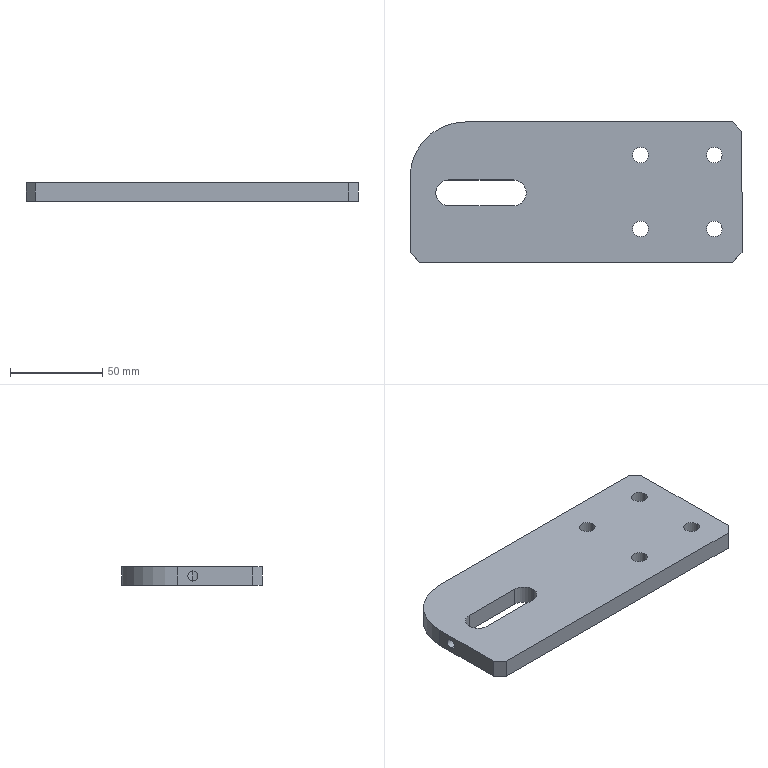Part | SolidWorks | features HoleWzd 2, Chamfer 1, Extrusion 1, ICE 1, LPattern 1, MirrorPattern 1 | 1 solid | 25 faces | box 180 x 76 x 10 mm | volume 125449 mm3 | cylinder 14 | plane 11 | commonest cylinder face diameters 8.5 x8 14 x3 5.5 x2 60 x1
STEP:
#1=CARTESIAN_POINT('',(-76.,-0.5,-2.75));
#2=VERTEX_POINT('',#1);
#3=CARTESIAN_POINT('',(-76.,-0.5,2.75));
#4=VERTEX_POINT('',#3);
#5=CARTESIAN_POINT('',(-76.,-0.5,-2.75));
#6=CARTESIAN_POINT('',(-76.,-0.6808,-2.75));
#7=CARTESIAN_POINT('',(-75.993,-0.8639,-2.732));
#8=CARTESIAN_POINT('',(-75.965,-1.22,-2.66));
#9=CARTESIAN_POINT('',(-75.945,-1.392,-2.607));
#10=CARTESIAN_POINT('',(-75.894,-1.725,-2.469));
#11=CARTESIAN_POINT('',(-75.863,-1.885,-2.382));
#12=CARTESIAN_POINT('',(-75.797,-2.181,-2.184));
#13=CARTESIAN_POINT('',(-75.761,-2.319,-2.071));
#14=CARTESIAN_POINT('',(-75.687,-2.572,-1.817));
#15=CARTESIAN_POINT('',(-75.651,-2.685,-1.679));
#16=CARTESIAN_POINT('',(-75.583,-2.883,-1.384));
#17=CARTESIAN_POINT('',(-75.551,-2.969,-1.224));
#18=CARTESIAN_POINT('',(-75.497,-3.107,-0.8921));
#19=CARTESIAN_POINT('',(-75.475,-3.16,-0.7207));
#20=CARTESIAN_POINT('',(-75.445,-3.231,-0.3666));
#21=CARTESIAN_POINT('',(-75.437,-3.25,-0.1823));
#22=CARTESIAN_POINT('',(-75.437,-3.25,0.18));
#23=CARTESIAN_POINT('',(-75.445,-3.232,0.3601));
#24=CARTESIAN_POINT('',(-75.475,-3.161,0.7177));
#25=CARTESIAN_POINT('',(-75.497,-3.108,0.8913));
#26=CARTESIAN_POINT('',(-75.55,-2.97,1.222));
#27=CARTESIAN_POINT('',(-75.582,-2.884,1.382));
#28=CARTESIAN_POINT('',(-75.651,-2.685,1.679));
#29=CARTESIAN_POINT('',(-75.688,-2.572,1.817));
#30=CARTESIAN_POINT('',(-75.76,-2.32,2.069));
#31=CARTESIAN_POINT('',(-75.797,-2.181,2.184));
#32=CARTESIAN_POINT('',(-75.863,-1.885,2.382));
#33=CARTESIAN_POINT('',(-75.893,-1.728,2.467));
#34=CARTESIAN_POINT('',(-75.97,-1.227,2.677));
#35=CARTESIAN_POINT('',(-76.,-0.8671,2.75));
#36=CARTESIAN_POINT('',(-76.,-0.5,2.75));
#37=B_SPLINE_CURVE_WITH_KNOTS('',3,(#5,#6,#7,#8,#9,#10,#11,#12,#13,#14,#15,#16,#17,#18,#19,#20,#21,#22,#23,#24,#25,#26,#27,#28,#29,#30,#31,#32,#33,#34,#35,#36),.UNSPECIFIED.,.F.,.F.,(4,2,2,2,2,2,2,2,2,2,2,2,2,2,2,4),(0.008686,0.009229,0.009771,0.01031,0.01086,0.0114,0.01194,0.01248,0.01303,0.01357,0.01411,0.01465,0.0152,0.01574,0.01628,0.01737),.UNSPECIFIED.);
#38=EDGE_CURVE('',#2,#4,#37,.T.);
#39=ORIENTED_EDGE('',*,*,#38,.F.);
#40=CARTESIAN_POINT('',(-90.,-0.5,-2.75));
#41=VERTEX_POINT('',#40);
#42=CARTESIAN_POINT('',(-90.,-0.5,-2.75));
#43=DIRECTION('',(-1.,0.,0.));
#44=VECTOR('',#43,1000.);
#45=LINE('',#42,#44);
#46=EDGE_CURVE('',#2,#41,#45,.T.);
#47=ORIENTED_EDGE('',*,*,#46,.T.);
#48=CARTESIAN_POINT('',(-90.,-0.5,2.75));
#49=VERTEX_POINT('',#48);
#50=CARTESIAN_POINT('',(-90.,-0.5,0.));
#51=DIRECTION('',(-1.,0.,0.));
#52=DIRECTION('',(0.,0.,1.));
#53=AXIS2_PLACEMENT_3D('',#50,#51,#52);
#54=CIRCLE('',#53,2.75);
#55=EDGE_CURVE('',#41,#49,#54,.T.);
#56=ORIENTED_EDGE('',*,*,#55,.T.);
#57=CARTESIAN_POINT('',(-90.,-0.5,2.75));
#58=DIRECTION('',(-1.,0.,0.));
#59=VECTOR('',#58,1000.);
#60=LINE('',#57,#59);
#61=EDGE_CURVE('',#4,#49,#60,.T.);
#62=ORIENTED_EDGE('',*,*,#61,.F.);
#63=EDGE_LOOP('',(#39,#47,#56,#62));
#64=FACE_OUTER_BOUND('',#63,.T.);
#65=CARTESIAN_POINT('',(-90.,-0.5,0.));
#66=DIRECTION('',(-1.,0.,0.));
#67=DIRECTION('',(0.,0.,1.));
#68=AXIS2_PLACEMENT_3D('',#65,#66,#67);
#69=CYLINDRICAL_SURFACE('',#68,2.75);
#70=ADVANCED_FACE('',(#64),#69,.F.);
#71=CARTESIAN_POINT('',(-27.,-0.5,-5.));
#72=VERTEX_POINT('',#71);
#73=CARTESIAN_POINT('',(-34.,6.5,-5.));
#74=VERTEX_POINT('',#73);
#75=CARTESIAN_POINT('',(-34.,-0.5,-5.));
#76=DIRECTION('',(0.,0.,1.));
#77=DIRECTION('',(1.,0.,0.));
#78=AXIS2_PLACEMENT_3D('',#75,#76,#77);
#79=CIRCLE('',#78,7.);
#80=EDGE_CURVE('',#72,#74,#79,.T.);
#81=ORIENTED_EDGE('',*,*,#80,.F.);
#82=CARTESIAN_POINT('',(-27.,-0.5,5.));
#83=VERTEX_POINT('',#82);
#84=CARTESIAN_POINT('',(-27.,-0.5,-5.));
#85=DIRECTION('',(0.,0.,1.));
#86=VECTOR('',#85,1000.);
#87=LINE('',#84,#86);
#88=EDGE_CURVE('',#72,#83,#87,.T.);
#89=ORIENTED_EDGE('',*,*,#88,.T.);
#90=CARTESIAN_POINT('',(-34.,6.5,5.));
#91=VERTEX_POINT('',#90);
#92=CARTESIAN_POINT('',(-34.,-0.5,5.));
#93=DIRECTION('',(0.,0.,1.));
#94=DIRECTION('',(1.,0.,0.));
#95=AXIS2_PLACEMENT_3D('',#92,#93,#94);
#96=CIRCLE('',#95,7.);
#97=EDGE_CURVE('',#83,#91,#96,.T.);
#98=ORIENTED_EDGE('',*,*,#97,.T.);
#99=CARTESIAN_POINT('',(-34.,6.5,-5.));
#100=DIRECTION('',(0.,0.,1.));
#101=VECTOR('',#100,1000.);
#102=LINE('',#99,#101);
#103=EDGE_CURVE('',#74,#91,#102,.T.);
#104=ORIENTED_EDGE('',*,*,#103,.F.);
#105=EDGE_LOOP('',(#81,#89,#98,#104));
#106=FACE_OUTER_BOUND('',#105,.T.);
#107=CARTESIAN_POINT('',(-34.,-0.5,-5.));
#108=DIRECTION('',(0.,0.,1.));
#109=DIRECTION('',(1.,0.,0.));
#110=AXIS2_PLACEMENT_3D('',#107,#108,#109);
#111=CYLINDRICAL_SURFACE('',#110,7.);
#112=ADVANCED_FACE('',(#106),#111,.F.);
#113=CARTESIAN_POINT('',(30.75,-20.,-5.));
#114=VERTEX_POINT('',#113);
#115=CARTESIAN_POINT('',(39.25,-20.,-5.));
#116=VERTEX_POINT('',#115);
#117=CARTESIAN_POINT('',(35.,-20.,-5.));
#118=DIRECTION('',(0.,0.,1.));
#119=DIRECTION('',(1.,0.,0.));
#120=AXIS2_PLACEMENT_3D('',#117,#118,#119);
#121=CIRCLE('',#120,4.25);
#122=EDGE_CURVE('',#114,#116,#121,.T.);
#123=ORIENTED_EDGE('',*,*,#122,.F.);
#124=CARTESIAN_POINT('',(30.75,-20.,5.));
#125=VERTEX_POINT('',#124);
#126=CARTESIAN_POINT('',(30.75,-20.,5.));
#127=DIRECTION('',(0.,0.,1.));
#128=VECTOR('',#127,1000.);
#129=LINE('',#126,#128);
#130=EDGE_CURVE('',#114,#125,#129,.T.);
#131=ORIENTED_EDGE('',*,*,#130,.T.);
#132=CARTESIAN_POINT('',(39.25,-20.,5.));
#133=VERTEX_POINT('',#132);
#134=CARTESIAN_POINT('',(35.,-20.,5.));
#135=DIRECTION('',(0.,0.,1.));
#136=DIRECTION('',(1.,0.,0.));
#137=AXIS2_PLACEMENT_3D('',#134,#135,#136);
#138=CIRCLE('',#137,4.25);
#139=EDGE_CURVE('',#125,#133,#138,.T.);
#140=ORIENTED_EDGE('',*,*,#139,.T.);
#141=CARTESIAN_POINT('',(39.25,-20.,5.));
#142=DIRECTION('',(0.,0.,1.));
#143=VECTOR('',#142,1000.);
#144=LINE('',#141,#143);
#145=EDGE_CURVE('',#116,#133,#144,.T.);
#146=ORIENTED_EDGE('',*,*,#145,.F.);
#147=EDGE_LOOP('',(#123,#131,#140,#146));
#148=FACE_OUTER_BOUND('',#147,.T.);
#149=CARTESIAN_POINT('',(35.,-20.,5.));
#150=DIRECTION('',(0.,0.,1.));
#151=DIRECTION('',(1.,0.,0.));
#152=AXIS2_PLACEMENT_3D('',#149,#150,#151);
#153=CYLINDRICAL_SURFACE('',#152,4.25);
#154=ADVANCED_FACE('',(#148),#153,.F.);
#155=CARTESIAN_POINT('',(70.75,-20.,-5.));
#156=VERTEX_POINT('',#155);
#157=CARTESIAN_POINT('',(79.25,-20.,-5.));
#158=VERTEX_POINT('',#157);
#159=CARTESIAN_POINT('',(75.,-20.,-5.));
#160=DIRECTION('',(0.,0.,1.));
#161=DIRECTION('',(1.,0.,0.));
#162=AXIS2_PLACEMENT_3D('',#159,#160,#161);
#163=CIRCLE('',#162,4.25);
#164=EDGE_CURVE('',#156,#158,#163,.T.);
#165=ORIENTED_EDGE('',*,*,#164,.F.);
#166=CARTESIAN_POINT('',(70.75,-20.,5.));
#167=VERTEX_POINT('',#166);
#168=CARTESIAN_POINT('',(70.75,-20.,5.));
#169=DIRECTION('',(0.,0.,1.));
#170=VECTOR('',#169,1000.);
#171=LINE('',#168,#170);
#172=EDGE_CURVE('',#156,#167,#171,.T.);
#173=ORIENTED_EDGE('',*,*,#172,.T.);
#174=CARTESIAN_POINT('',(79.25,-20.,5.));
#175=VERTEX_POINT('',#174);
#176=CARTESIAN_POINT('',(75.,-20.,5.));
#177=DIRECTION('',(0.,0.,1.));
#178=DIRECTION('',(1.,0.,0.));
#179=AXIS2_PLACEMENT_3D('',#176,#177,#178);
#180=CIRCLE('',#179,4.25);
#181=EDGE_CURVE('',#167,#175,#180,.T.);
#182=ORIENTED_EDGE('',*,*,#181,.T.);
#183=CARTESIAN_POINT('',(79.25,-20.,5.));
#184=DIRECTION('',(0.,0.,1.));
#185=VECTOR('',#184,1000.);
#186=LINE('',#183,#185);
#187=EDGE_CURVE('',#158,#175,#186,.T.);
#188=ORIENTED_EDGE('',*,*,#187,.F.);
#189=EDGE_LOOP('',(#165,#173,#182,#188));
#190=FACE_OUTER_BOUND('',#189,.T.);
#191=CARTESIAN_POINT('',(75.,-20.,5.));
#192=DIRECTION('',(0.,0.,1.));
#193=DIRECTION('',(1.,0.,0.));
#194=AXIS2_PLACEMENT_3D('',#191,#192,#193);
#195=CYLINDRICAL_SURFACE('',#194,4.25);
#196=ADVANCED_FACE('',(#190),#195,.F.);
#197=CARTESIAN_POINT('',(30.75,20.,-5.));
#198=VERTEX_POINT('',#197);
#199=CARTESIAN_POINT('',(39.25,20.,-5.));
#200=VERTEX_POINT('',#199);
#201=CARTESIAN_POINT('',(35.,20.,-5.));
#202=DIRECTION('',(0.,0.,1.));
#203=DIRECTION('',(1.,0.,0.));
#204=AXIS2_PLACEMENT_3D('',#201,#202,#203);
#205=CIRCLE('',#204,4.25);
#206=EDGE_CURVE('',#198,#200,#205,.T.);
#207=ORIENTED_EDGE('',*,*,#206,.F.);
#208=CARTESIAN_POINT('',(30.75,20.,5.));
#209=VERTEX_POINT('',#208);
#210=CARTESIAN_POINT('',(30.75,20.,5.));
#211=DIRECTION('',(0.,0.,1.));
#212=VECTOR('',#211,1000.);
#213=LINE('',#210,#212);
#214=EDGE_CURVE('',#198,#209,#213,.T.);
#215=ORIENTED_EDGE('',*,*,#214,.T.);
#216=CARTESIAN_POINT('',(39.25,20.,5.));
#217=VERTEX_POINT('',#216);
#218=CARTESIAN_POINT('',(35.,20.,5.));
#219=DIRECTION('',(0.,0.,1.));
#220=DIRECTION('',(1.,0.,0.));
#221=AXIS2_PLACEMENT_3D('',#218,#219,#220);
#222=CIRCLE('',#221,4.25);
#223=EDGE_CURVE('',#209,#217,#222,.T.);
#224=ORIENTED_EDGE('',*,*,#223,.T.);
#225=CARTESIAN_POINT('',(39.25,20.,5.));
#226=DIRECTION('',(0.,0.,1.));
#227=VECTOR('',#226,1000.);
#228=LINE('',#225,#227);
#229=EDGE_CURVE('',#200,#217,#228,.T.);
#230=ORIENTED_EDGE('',*,*,#229,.F.);
#231=EDGE_LOOP('',(#207,#215,#224,#230));
#232=FACE_OUTER_BOUND('',#231,.T.);
#233=CARTESIAN_POINT('',(35.,20.,5.));
#234=DIRECTION('',(0.,0.,1.));
#235=DIRECTION('',(1.,0.,0.));
#236=AXIS2_PLACEMENT_3D('',#233,#234,#235);
#237=CYLINDRICAL_SURFACE('',#236,4.25);
#238=ADVANCED_FACE('',(#232),#237,.F.);
#239=CARTESIAN_POINT('',(70.75,20.,-5.));
#240=VERTEX_POINT('',#239);
#241=CARTESIAN_POINT('',(79.25,20.,-5.));
#242=VERTEX_POINT('',#241);
#243=CARTESIAN_POINT('',(75.,20.,-5.));
#244=DIRECTION('',(0.,0.,1.));
#245=DIRECTION('',(1.,0.,0.));
#246=AXIS2_PLACEMENT_3D('',#243,#244,#245);
#247=CIRCLE('',#246,4.25);
#248=EDGE_CURVE('',#240,#242,#247,.T.);
#249=ORIENTED_EDGE('',*,*,#248,.F.);
#250=CARTESIAN_POINT('',(70.75,20.,5.));
#251=VERTEX_POINT('',#250);
#252=CARTESIAN_POINT('',(70.75,20.,5.));
#253=DIRECTION('',(0.,0.,1.));
#254=VECTOR('',#253,1000.);
#255=LINE('',#252,#254);
#256=EDGE_CURVE('',#240,#251,#255,.T.);
#257=ORIENTED_EDGE('',*,*,#256,.T.);
#258=CARTESIAN_POINT('',(79.25,20.,5.));
#259=VERTEX_POINT('',#258);
#260=CARTESIAN_POINT('',(75.,20.,5.));
#261=DIRECTION('',(0.,0.,1.));
#262=DIRECTION('',(1.,0.,0.));
#263=AXIS2_PLACEMENT_3D('',#260,#261,#262);
#264=CIRCLE('',#263,4.25);
#265=EDGE_CURVE('',#251,#259,#264,.T.);
#266=ORIENTED_EDGE('',*,*,#265,.T.);
#267=CARTESIAN_POINT('',(79.25,20.,5.));
#268=DIRECTION('',(0.,0.,1.));
#269=VECTOR('',#268,1000.);
#270=LINE('',#267,#269);
#271=EDGE_CURVE('',#242,#259,#270,.T.);
#272=ORIENTED_EDGE('',*,*,#271,.F.);
#273=EDGE_LOOP('',(#249,#257,#266,#272));
#274=FACE_OUTER_BOUND('',#273,.T.);
#275=CARTESIAN_POINT('',(75.,20.,5.));
#276=DIRECTION('',(0.,0.,1.));
#277=DIRECTION('',(1.,0.,0.));
#278=AXIS2_PLACEMENT_3D('',#275,#276,#277);
#279=CYLINDRICAL_SURFACE('',#278,4.25);
#280=ADVANCED_FACE('',(#274),#279,.F.);
#281=CARTESIAN_POINT('',(90.,-33.,-5.));
#282=VERTEX_POINT('',#281);
#283=CARTESIAN_POINT('',(90.,33.,-5.));
#284=VERTEX_POINT('',#283);
#285=CARTESIAN_POINT('',(90.,38.,-5.));
#286=DIRECTION('',(0.,1.,0.));
#287=VECTOR('',#286,1000.);
#288=LINE('',#285,#287);
#289=EDGE_CURVE('',#282,#284,#288,.T.);
#290=ORIENTED_EDGE('',*,*,#289,.T.);
#291=CARTESIAN_POINT('',(90.,33.,5.));
#292=VERTEX_POINT('',#291);
#293=CARTESIAN_POINT('',(90.,33.,5.));
#294=DIRECTION('',(0.,0.,1.));
#295=VECTOR('',#294,1000.);
#296=LINE('',#293,#295);
#297=EDGE_CURVE('',#284,#292,#296,.T.);
#298=ORIENTED_EDGE('',*,*,#297,.T.);
#299=CARTESIAN_POINT('',(90.,-33.,5.));
#300=VERTEX_POINT('',#299);
#301=CARTESIAN_POINT('',(90.,38.,5.));
#302=DIRECTION('',(0.,1.,0.));
#303=VECTOR('',#302,1000.);
#304=LINE('',#301,#303);
#305=EDGE_CURVE('',#300,#292,#304,.T.);
#306=ORIENTED_EDGE('',*,*,#305,.F.);
#307=CARTESIAN_POINT('',(90.,-33.,5.));
#308=DIRECTION('',(0.,0.,-1.));
#309=VECTOR('',#308,1000.);
#310=LINE('',#307,#309);
#311=EDGE_CURVE('',#300,#282,#310,.T.);
#312=ORIENTED_EDGE('',*,*,#311,.T.);
#313=EDGE_LOOP('',(#290,#298,#306,#312));
#314=FACE_OUTER_BOUND('',#313,.T.);
#315=CARTESIAN_POINT('',(90.,38.,5.));
#316=DIRECTION('',(-1.,0.,0.));
#317=DIRECTION('',(0.,-1.,0.));
#318=AXIS2_PLACEMENT_3D('',#315,#316,#317);
#319=PLANE('',#318);
#320=ADVANCED_FACE('',(#314),#319,.F.);
#321=CARTESIAN_POINT('',(85.,38.,5.));
#322=VERTEX_POINT('',#321);
#323=CARTESIAN_POINT('',(-60.,38.,5.));
#324=VERTEX_POINT('',#323);
#325=CARTESIAN_POINT('',(-60.,38.,5.));
#326=DIRECTION('',(-1.,0.,0.));
#327=VECTOR('',#326,1000.);
#328=LINE('',#325,#327);
#329=EDGE_CURVE('',#322,#324,#328,.T.);
#330=ORIENTED_EDGE('',*,*,#329,.F.);
#331=CARTESIAN_POINT('',(85.,38.,-5.));
#332=VERTEX_POINT('',#331);
#333=CARTESIAN_POINT('',(85.,38.,5.));
#334=DIRECTION('',(0.,0.,-1.));
#335=VECTOR('',#334,1000.);
#336=LINE('',#333,#335);
#337=EDGE_CURVE('',#322,#332,#336,.T.);
#338=ORIENTED_EDGE('',*,*,#337,.T.);
#339=CARTESIAN_POINT('',(-60.,38.,-5.));
#340=VERTEX_POINT('',#339);
#341=CARTESIAN_POINT('',(-60.,38.,-5.));
#342=DIRECTION('',(-1.,0.,0.));
#343=VECTOR('',#342,1000.);
#344=LINE('',#341,#343);
#345=EDGE_CURVE('',#332,#340,#344,.T.);
#346=ORIENTED_EDGE('',*,*,#345,.T.);
#347=CARTESIAN_POINT('',(-60.,38.,5.));
#348=DIRECTION('',(0.,0.,-1.));
#349=VECTOR('',#348,1000.);
#350=LINE('',#347,#349);
#351=EDGE_CURVE('',#324,#340,#350,.T.);
#352=ORIENTED_EDGE('',*,*,#351,.F.);
#353=EDGE_LOOP('',(#330,#338,#346,#352));
#354=FACE_OUTER_BOUND('',#353,.T.);
#355=CARTESIAN_POINT('',(-60.,38.,5.));
#356=DIRECTION('',(0.,-1.,0.));
#357=DIRECTION('',(0.,0.,-1.));
#358=AXIS2_PLACEMENT_3D('',#355,#356,#357);
#359=PLANE('',#358);
#360=ADVANCED_FACE('',(#354),#359,.F.);
#361=CARTESIAN_POINT('',(-90.,8.,-5.));
#362=VERTEX_POINT('',#361);
#363=CARTESIAN_POINT('',(-60.,8.,-5.));
#364=DIRECTION('',(0.,0.,1.));
#365=DIRECTION('',(-1.,0.,0.));
#366=AXIS2_PLACEMENT_3D('',#363,#364,#365);
#367=CIRCLE('',#366,30.);
#368=EDGE_CURVE('',#340,#362,#367,.T.);
#369=ORIENTED_EDGE('',*,*,#368,.T.);
#370=CARTESIAN_POINT('',(-90.,8.,5.));
#371=VERTEX_POINT('',#370);
#372=CARTESIAN_POINT('',(-90.,8.,5.));
#373=DIRECTION('',(0.,0.,-1.));
#374=VECTOR('',#373,1000.);
#375=LINE('',#372,#374);
#376=EDGE_CURVE('',#371,#362,#375,.T.);
#377=ORIENTED_EDGE('',*,*,#376,.F.);
#378=CARTESIAN_POINT('',(-60.,8.,5.));
#379=DIRECTION('',(0.,0.,1.));
#380=DIRECTION('',(-1.,0.,0.));
#381=AXIS2_PLACEMENT_3D('',#378,#379,#380);
#382=CIRCLE('',#381,30.);
#383=EDGE_CURVE('',#324,#371,#382,.T.);
#384=ORIENTED_EDGE('',*,*,#383,.F.);
#385=ORIENTED_EDGE('',*,*,#351,.T.);
#386=EDGE_LOOP('',(#369,#377,#384,#385));
#387=FACE_OUTER_BOUND('',#386,.T.);
#388=CARTESIAN_POINT('',(-60.,8.,5.));
#389=DIRECTION('',(0.,0.,-1.));
#390=DIRECTION('',(-1.,0.,0.));
#391=AXIS2_PLACEMENT_3D('',#388,#389,#390);
#392=CYLINDRICAL_SURFACE('',#391,30.);
#393=ADVANCED_FACE('',(#387),#392,.T.);
#394=CARTESIAN_POINT('',(-90.,-0.5,0.));
#395=DIRECTION('',(-1.,0.,0.));
#396=DIRECTION('',(0.,0.,1.));
#397=AXIS2_PLACEMENT_3D('',#394,#395,#396);
#398=CIRCLE('',#397,2.75);
#399=EDGE_CURVE('',#49,#41,#398,.T.);
#400=ORIENTED_EDGE('',*,*,#399,.F.);
#401=ORIENTED_EDGE('',*,*,#55,.F.);
#402=EDGE_LOOP('',(#400,#401));
#403=FACE_BOUND('',#402,.T.);
#404=CARTESIAN_POINT('',(-90.,-33.,-5.));
#405=VERTEX_POINT('',#404);
#406=CARTESIAN_POINT('',(-90.,8.,-5.));
#407=DIRECTION('',(0.,-1.,0.));
#408=VECTOR('',#407,1000.);
#409=LINE('',#406,#408);
#410=EDGE_CURVE('',#362,#405,#409,.T.);
#411=ORIENTED_EDGE('',*,*,#410,.T.);
#412=CARTESIAN_POINT('',(-90.,-33.,5.));
#413=VERTEX_POINT('',#412);
#414=CARTESIAN_POINT('',(-90.,-33.,5.));
#415=DIRECTION('',(0.,0.,1.));
#416=VECTOR('',#415,1000.);
#417=LINE('',#414,#416);
#418=EDGE_CURVE('',#405,#413,#417,.T.);
#419=ORIENTED_EDGE('',*,*,#418,.T.);
#420=CARTESIAN_POINT('',(-90.,8.,5.));
#421=DIRECTION('',(0.,-1.,0.));
#422=VECTOR('',#421,1000.);
#423=LINE('',#420,#422);
#424=EDGE_CURVE('',#371,#413,#423,.T.);
#425=ORIENTED_EDGE('',*,*,#424,.F.);
#426=ORIENTED_EDGE('',*,*,#376,.T.);
#427=EDGE_LOOP('',(#411,#419,#425,#426));
#428=FACE_OUTER_BOUND('',#427,.T.);
#429=CARTESIAN_POINT('',(-90.,8.,5.));
#430=DIRECTION('',(1.,0.,0.));
#431=DIRECTION('',(0.,1.,0.));
#432=AXIS2_PLACEMENT_3D('',#429,#430,#431);
#433=PLANE('',#432);
#434=ADVANCED_FACE('',(#403,#428),#433,.F.);
#435=CARTESIAN_POINT('',(-85.,-38.,-5.));
#436=VERTEX_POINT('',#435);
#437=CARTESIAN_POINT('',(85.,-38.,-5.));
#438=VERTEX_POINT('',#437);
#439=CARTESIAN_POINT('',(-90.,-38.,-5.));
#440=DIRECTION('',(1.,0.,0.));
#441=VECTOR('',#440,1000.);
#442=LINE('',#439,#441);
#443=EDGE_CURVE('',#436,#438,#442,.T.);
#444=ORIENTED_EDGE('',*,*,#443,.T.);
#445=CARTESIAN_POINT('',(85.,-38.,5.));
#446=VERTEX_POINT('',#445);
#447=CARTESIAN_POINT('',(85.,-38.,5.));
#448=DIRECTION('',(0.,0.,1.));
#449=VECTOR('',#448,1000.);
#450=LINE('',#447,#449);
#451=EDGE_CURVE('',#438,#446,#450,.T.);
#452=ORIENTED_EDGE('',*,*,#451,.T.);
#453=CARTESIAN_POINT('',(-85.,-38.,5.));
#454=VERTEX_POINT('',#453);
#455=CARTESIAN_POINT('',(-90.,-38.,5.));
#456=DIRECTION('',(1.,0.,0.));
#457=VECTOR('',#456,1000.);
#458=LINE('',#455,#457);
#459=EDGE_CURVE('',#454,#446,#458,.T.);
#460=ORIENTED_EDGE('',*,*,#459,.F.);
#461=CARTESIAN_POINT('',(-85.,-38.,5.));
#462=DIRECTION('',(0.,0.,-1.));
#463=VECTOR('',#462,1000.);
#464=LINE('',#461,#463);
#465=EDGE_CURVE('',#454,#436,#464,.T.);
#466=ORIENTED_EDGE('',*,*,#465,.T.);
#467=EDGE_LOOP('',(#444,#452,#460,#466));
#468=FACE_OUTER_BOUND('',#467,.T.);
#469=CARTESIAN_POINT('',(-90.,-38.,5.));
#470=DIRECTION('',(0.,1.,0.));
#471=DIRECTION('',(0.,0.,1.));
#472=AXIS2_PLACEMENT_3D('',#469,#470,#471);
#473=PLANE('',#472);
#474=ADVANCED_FACE('',(#468),#473,.F.);
#475=CARTESIAN_POINT('',(-69.,-7.5,5.));
#476=VERTEX_POINT('',#475);
#477=CARTESIAN_POINT('',(-34.,-7.5,5.));
#478=VERTEX_POINT('',#477);
#479=CARTESIAN_POINT('',(-69.,-7.5,5.));
#480=DIRECTION('',(1.,0.,0.));
#481=VECTOR('',#480,1000.);
#482=LINE('',#479,#481);
#483=EDGE_CURVE('',#476,#478,#482,.T.);
#484=ORIENTED_EDGE('',*,*,#483,.F.);
#485=CARTESIAN_POINT('',(-69.,6.5,5.));
#486=VERTEX_POINT('',#485);
#487=CARTESIAN_POINT('',(-69.,-0.5,5.));
#488=DIRECTION('',(0.,0.,1.));
#489=DIRECTION('',(1.,0.,0.));
#490=AXIS2_PLACEMENT_3D('',#487,#488,#489);
#491=CIRCLE('',#490,7.);
#492=EDGE_CURVE('',#486,#476,#491,.T.);
#493=ORIENTED_EDGE('',*,*,#492,.F.);
#494=CARTESIAN_POINT('',(-69.,6.5,5.));
#495=DIRECTION('',(-1.,0.,0.));
#496=VECTOR('',#495,1000.);
#497=LINE('',#494,#496);
#498=EDGE_CURVE('',#91,#486,#497,.T.);
#499=ORIENTED_EDGE('',*,*,#498,.F.);
#500=ORIENTED_EDGE('',*,*,#97,.F.);
#501=CARTESIAN_POINT('',(-34.,-0.5,5.));
#502=DIRECTION('',(0.,0.,1.));
#503=DIRECTION('',(1.,0.,0.));
#504=AXIS2_PLACEMENT_3D('',#501,#502,#503);
#505=CIRCLE('',#504,7.);
#506=EDGE_CURVE('',#478,#83,#505,.T.);
#507=ORIENTED_EDGE('',*,*,#506,.F.);
#508=EDGE_LOOP('',(#484,#493,#499,#500,#507));
#509=FACE_BOUND('',#508,.T.);
#510=CARTESIAN_POINT('',(35.,-20.,5.));
#511=DIRECTION('',(0.,0.,1.));
#512=DIRECTION('',(1.,0.,0.));
#513=AXIS2_PLACEMENT_3D('',#510,#511,#512);
#514=CIRCLE('',#513,4.25);
#515=EDGE_CURVE('',#133,#125,#514,.T.);
#516=ORIENTED_EDGE('',*,*,#515,.F.);
#517=ORIENTED_EDGE('',*,*,#139,.F.);
#518=EDGE_LOOP('',(#516,#517));
#519=FACE_BOUND('',#518,.T.);
#520=CARTESIAN_POINT('',(75.,-20.,5.));
#521=DIRECTION('',(0.,0.,1.));
#522=DIRECTION('',(1.,0.,0.));
#523=AXIS2_PLACEMENT_3D('',#520,#521,#522);
#524=CIRCLE('',#523,4.25);
#525=EDGE_CURVE('',#175,#167,#524,.T.);
#526=ORIENTED_EDGE('',*,*,#525,.F.);
#527=ORIENTED_EDGE('',*,*,#181,.F.);
#528=EDGE_LOOP('',(#526,#527));
#529=FACE_BOUND('',#528,.T.);
#530=CARTESIAN_POINT('',(35.,20.,5.));
#531=DIRECTION('',(0.,0.,1.));
#532=DIRECTION('',(1.,0.,0.));
#533=AXIS2_PLACEMENT_3D('',#530,#531,#532);
#534=CIRCLE('',#533,4.25);
#535=EDGE_CURVE('',#217,#209,#534,.T.);
#536=ORIENTED_EDGE('',*,*,#535,.F.);
#537=ORIENTED_EDGE('',*,*,#223,.F.);
#538=EDGE_LOOP('',(#536,#537));
#539=FACE_BOUND('',#538,.T.);
#540=CARTESIAN_POINT('',(75.,20.,5.));
#541=DIRECTION('',(0.,0.,1.));
#542=DIRECTION('',(1.,0.,0.));
#543=AXIS2_PLACEMENT_3D('',#540,#541,#542);
#544=CIRCLE('',#543,4.25);
#545=EDGE_CURVE('',#259,#251,#544,.T.);
#546=ORIENTED_EDGE('',*,*,#545,.F.);
#547=ORIENTED_EDGE('',*,*,#265,.F.);
#548=EDGE_LOOP('',(#546,#547));
#549=FACE_BOUND('',#548,.T.);
#550=ORIENTED_EDGE('',*,*,#305,.T.);
#551=CARTESIAN_POINT('',(85.,38.,5.));
#552=DIRECTION('',(-0.7071,0.7071,0.));
#553=VECTOR('',#552,1000.);
#554=LINE('',#551,#553);
#555=EDGE_CURVE('',#292,#322,#554,.T.);
#556=ORIENTED_EDGE('',*,*,#555,.T.);
#557=ORIENTED_EDGE('',*,*,#329,.T.);
#558=ORIENTED_EDGE('',*,*,#383,.T.);
#559=ORIENTED_EDGE('',*,*,#424,.T.);
#560=CARTESIAN_POINT('',(-85.,-38.,5.));
#561=DIRECTION('',(0.7071,-0.7071,0.));
#562=VECTOR('',#561,1000.);
#563=LINE('',#560,#562);
#564=EDGE_CURVE('',#413,#454,#563,.T.);
#565=ORIENTED_EDGE('',*,*,#564,.T.);
#566=ORIENTED_EDGE('',*,*,#459,.T.);
#567=CARTESIAN_POINT('',(90.,-33.,5.));
#568=DIRECTION('',(0.7071,0.7071,0.));
#569=VECTOR('',#568,1000.);
#570=LINE('',#567,#569);
#571=EDGE_CURVE('',#446,#300,#570,.T.);
#572=ORIENTED_EDGE('',*,*,#571,.T.);
#573=EDGE_LOOP('',(#550,#556,#557,#558,#559,#565,#566,#572));
#574=FACE_OUTER_BOUND('',#573,.T.);
#575=CARTESIAN_POINT('',(-60.,8.,5.));
#576=DIRECTION('',(0.,0.,-1.));
#577=DIRECTION('',(-1.,0.,0.));
#578=AXIS2_PLACEMENT_3D('',#575,#576,#577);
#579=PLANE('',#578);
#580=ADVANCED_FACE('',(#509,#519,#529,#539,#549,#574),#579,.F.);
#581=CARTESIAN_POINT('',(-69.,6.5,-5.));
#582=VERTEX_POINT('',#581);
#583=CARTESIAN_POINT('',(-69.,-7.5,-5.));
#584=VERTEX_POINT('',#583);
#585=CARTESIAN_POINT('',(-69.,-0.5,-5.));
#586=DIRECTION('',(0.,0.,1.));
#587=DIRECTION('',(1.,0.,0.));
#588=AXIS2_PLACEMENT_3D('',#585,#586,#587);
#589=CIRCLE('',#588,7.);
#590=EDGE_CURVE('',#582,#584,#589,.T.);
#591=ORIENTED_EDGE('',*,*,#590,.T.);
#592=CARTESIAN_POINT('',(-34.,-7.5,-5.));
#593=VERTEX_POINT('',#592);
#594=CARTESIAN_POINT('',(-69.,-7.5,-5.));
#595=DIRECTION('',(1.,0.,0.));
#596=VECTOR('',#595,1000.);
#597=LINE('',#594,#596);
#598=EDGE_CURVE('',#584,#593,#597,.T.);
#599=ORIENTED_EDGE('',*,*,#598,.T.);
#600=CARTESIAN_POINT('',(-34.,-0.5,-5.));
#601=DIRECTION('',(0.,0.,1.));
#602=DIRECTION('',(1.,0.,0.));
#603=AXIS2_PLACEMENT_3D('',#600,#601,#602);
#604=CIRCLE('',#603,7.);
#605=EDGE_CURVE('',#593,#72,#604,.T.);
#606=ORIENTED_EDGE('',*,*,#605,.T.);
#607=ORIENTED_EDGE('',*,*,#80,.T.);
#608=CARTESIAN_POINT('',(-69.,6.5,-5.));
#609=DIRECTION('',(-1.,0.,0.));
#610=VECTOR('',#609,1000.);
#611=LINE('',#608,#610);
#612=EDGE_CURVE('',#74,#582,#611,.T.);
#613=ORIENTED_EDGE('',*,*,#612,.T.);
#614=EDGE_LOOP('',(#591,#599,#606,#607,#613));
#615=FACE_BOUND('',#614,.T.);
#616=CARTESIAN_POINT('',(35.,-20.,-5.));
#617=DIRECTION('',(0.,0.,1.));
#618=DIRECTION('',(1.,0.,0.));
#619=AXIS2_PLACEMENT_3D('',#616,#617,#618);
#620=CIRCLE('',#619,4.25);
#621=EDGE_CURVE('',#116,#114,#620,.T.);
#622=ORIENTED_EDGE('',*,*,#621,.T.);
#623=ORIENTED_EDGE('',*,*,#122,.T.);
#624=EDGE_LOOP('',(#622,#623));
#625=FACE_BOUND('',#624,.T.);
#626=CARTESIAN_POINT('',(75.,-20.,-5.));
#627=DIRECTION('',(0.,0.,1.));
#628=DIRECTION('',(1.,0.,0.));
#629=AXIS2_PLACEMENT_3D('',#626,#627,#628);
#630=CIRCLE('',#629,4.25);
#631=EDGE_CURVE('',#158,#156,#630,.T.);
#632=ORIENTED_EDGE('',*,*,#631,.T.);
#633=ORIENTED_EDGE('',*,*,#164,.T.);
#634=EDGE_LOOP('',(#632,#633));
#635=FACE_BOUND('',#634,.T.);
#636=CARTESIAN_POINT('',(35.,20.,-5.));
#637=DIRECTION('',(0.,0.,1.));
#638=DIRECTION('',(1.,0.,0.));
#639=AXIS2_PLACEMENT_3D('',#636,#637,#638);
#640=CIRCLE('',#639,4.25);
#641=EDGE_CURVE('',#200,#198,#640,.T.);
#642=ORIENTED_EDGE('',*,*,#641,.T.);
#643=ORIENTED_EDGE('',*,*,#206,.T.);
#644=EDGE_LOOP('',(#642,#643));
#645=FACE_BOUND('',#644,.T.);
#646=CARTESIAN_POINT('',(75.,20.,-5.));
#647=DIRECTION('',(0.,0.,1.));
#648=DIRECTION('',(1.,0.,0.));
#649=AXIS2_PLACEMENT_3D('',#646,#647,#648);
#650=CIRCLE('',#649,4.25);
#651=EDGE_CURVE('',#242,#240,#650,.T.);
#652=ORIENTED_EDGE('',*,*,#651,.T.);
#653=ORIENTED_EDGE('',*,*,#248,.T.);
#654=EDGE_LOOP('',(#652,#653));
#655=FACE_BOUND('',#654,.T.);
#656=ORIENTED_EDGE('',*,*,#345,.F.);
#657=CARTESIAN_POINT('',(27.5,95.5,-5.));
#658=DIRECTION('',(0.7071,-0.7071,0.));
#659=VECTOR('',#658,1000.);
#660=LINE('',#657,#659);
#661=EDGE_CURVE('',#332,#284,#660,.T.);
#662=ORIENTED_EDGE('',*,*,#661,.T.);
#663=ORIENTED_EDGE('',*,*,#289,.F.);
#664=CARTESIAN_POINT('',(35.5,-87.5,-5.));
#665=DIRECTION('',(-0.7071,-0.7071,0.));
#666=VECTOR('',#665,1000.);
#667=LINE('',#664,#666);
#668=EDGE_CURVE('',#282,#438,#667,.T.);
#669=ORIENTED_EDGE('',*,*,#668,.T.);
#670=ORIENTED_EDGE('',*,*,#443,.F.);
#671=CARTESIAN_POINT('',(-95.5,-27.5,-5.));
#672=DIRECTION('',(-0.7071,0.7071,0.));
#673=VECTOR('',#672,1000.);
#674=LINE('',#671,#673);
#675=EDGE_CURVE('',#436,#405,#674,.T.);
#676=ORIENTED_EDGE('',*,*,#675,.T.);
#677=ORIENTED_EDGE('',*,*,#410,.F.);
#678=ORIENTED_EDGE('',*,*,#368,.F.);
#679=EDGE_LOOP('',(#656,#662,#663,#669,#670,#676,#677,#678));
#680=FACE_OUTER_BOUND('',#679,.T.);
#681=CARTESIAN_POINT('',(-60.,8.,-5.));
#682=DIRECTION('',(0.,0.,-1.));
#683=DIRECTION('',(-1.,0.,0.));
#684=AXIS2_PLACEMENT_3D('',#681,#682,#683);
#685=PLANE('',#684);
#686=ADVANCED_FACE('',(#615,#625,#635,#645,#655,#680),#685,.T.);
#687=ORIENTED_EDGE('',*,*,#256,.F.);
#688=ORIENTED_EDGE('',*,*,#651,.F.);
#689=ORIENTED_EDGE('',*,*,#271,.T.);
#690=ORIENTED_EDGE('',*,*,#545,.T.);
#691=EDGE_LOOP('',(#687,#688,#689,#690));
#692=FACE_OUTER_BOUND('',#691,.T.);
#693=CARTESIAN_POINT('',(75.,20.,5.));
#694=DIRECTION('',(0.,0.,1.));
#695=DIRECTION('',(1.,0.,0.));
#696=AXIS2_PLACEMENT_3D('',#693,#694,#695);
#697=CYLINDRICAL_SURFACE('',#696,4.25);
#698=ADVANCED_FACE('',(#692),#697,.F.);
#699=ORIENTED_EDGE('',*,*,#214,.F.);
#700=ORIENTED_EDGE('',*,*,#641,.F.);
#701=ORIENTED_EDGE('',*,*,#229,.T.);
#702=ORIENTED_EDGE('',*,*,#535,.T.);
#703=EDGE_LOOP('',(#699,#700,#701,#702));
#704=FACE_OUTER_BOUND('',#703,.T.);
#705=CARTESIAN_POINT('',(35.,20.,5.));
#706=DIRECTION('',(0.,0.,1.));
#707=DIRECTION('',(1.,0.,0.));
#708=AXIS2_PLACEMENT_3D('',#705,#706,#707);
#709=CYLINDRICAL_SURFACE('',#708,4.25);
#710=ADVANCED_FACE('',(#704),#709,.F.);
#711=ORIENTED_EDGE('',*,*,#172,.F.);
#712=ORIENTED_EDGE('',*,*,#631,.F.);
#713=ORIENTED_EDGE('',*,*,#187,.T.);
#714=ORIENTED_EDGE('',*,*,#525,.T.);
#715=EDGE_LOOP('',(#711,#712,#713,#714));
#716=FACE_OUTER_BOUND('',#715,.T.);
#717=CARTESIAN_POINT('',(75.,-20.,5.));
#718=DIRECTION('',(0.,0.,1.));
#719=DIRECTION('',(1.,0.,0.));
#720=AXIS2_PLACEMENT_3D('',#717,#718,#719);
#721=CYLINDRICAL_SURFACE('',#720,4.25);
#722=ADVANCED_FACE('',(#716),#721,.F.);
#723=ORIENTED_EDGE('',*,*,#130,.F.);
#724=ORIENTED_EDGE('',*,*,#621,.F.);
#725=ORIENTED_EDGE('',*,*,#145,.T.);
#726=ORIENTED_EDGE('',*,*,#515,.T.);
#727=EDGE_LOOP('',(#723,#724,#725,#726));
#728=FACE_OUTER_BOUND('',#727,.T.);
#729=CARTESIAN_POINT('',(35.,-20.,5.));
#730=DIRECTION('',(0.,0.,1.));
#731=DIRECTION('',(1.,0.,0.));
#732=AXIS2_PLACEMENT_3D('',#729,#730,#731);
#733=CYLINDRICAL_SURFACE('',#732,4.25);
#734=ADVANCED_FACE('',(#728),#733,.F.);
#735=CARTESIAN_POINT('',(-76.,-0.5,2.75));
#736=CARTESIAN_POINT('',(-76.,-0.3163,2.75));
#737=CARTESIAN_POINT('',(-75.993,-0.136,2.732));
#738=CARTESIAN_POINT('',(-75.965,0.2181,2.661));
#739=CARTESIAN_POINT('',(-75.945,0.3938,2.607));
#740=CARTESIAN_POINT('',(-75.894,0.7261,2.468));
#741=CARTESIAN_POINT('',(-75.864,0.8834,2.383));
#742=CARTESIAN_POINT('',(-75.797,1.181,2.184));
#743=CARTESIAN_POINT('',(-75.76,1.32,2.069));
#744=CARTESIAN_POINT('',(-75.652,1.697,1.692));
#745=CARTESIAN_POINT('',(-75.577,1.9,1.389));
#746=CARTESIAN_POINT('',(-75.497,2.107,0.8938));
#747=CARTESIAN_POINT('',(-75.475,2.161,0.7186));
#748=CARTESIAN_POINT('',(-75.445,2.232,0.3628));
#749=CARTESIAN_POINT('',(-75.437,2.25,0.1831));
#750=CARTESIAN_POINT('',(-75.437,2.25,-0.1798));
#751=CARTESIAN_POINT('',(-75.445,2.232,-0.3641));
#752=CARTESIAN_POINT('',(-75.475,2.161,-0.7185));
#753=CARTESIAN_POINT('',(-75.496,2.108,-0.891));
#754=CARTESIAN_POINT('',(-75.551,1.968,-1.226));
#755=CARTESIAN_POINT('',(-75.583,1.883,-1.384));
#756=CARTESIAN_POINT('',(-75.651,1.685,-1.68));
#757=CARTESIAN_POINT('',(-75.688,1.57,-1.819));
#758=CARTESIAN_POINT('',(-75.761,1.318,-2.071));
#759=CARTESIAN_POINT('',(-75.797,1.181,-2.184));
#760=CARTESIAN_POINT('',(-75.864,0.8836,-2.383));
#761=CARTESIAN_POINT('',(-75.894,0.7232,-2.469));
#762=CARTESIAN_POINT('',(-75.945,0.3926,-2.607));
#763=CARTESIAN_POINT('',(-75.965,0.2207,-2.66));
#764=CARTESIAN_POINT('',(-75.993,-0.1374,-2.732));
#765=CARTESIAN_POINT('',(-76.,-0.3191,-2.75));
#766=CARTESIAN_POINT('',(-76.,-0.5,-2.75));
#767=B_SPLINE_CURVE_WITH_KNOTS('',3,(#735,#736,#737,#738,#739,#740,#741,#742,#743,#744,#745,#746,#747,#748,#749,#750,#751,#752,#753,#754,#755,#756,#757,#758,#759,#760,#761,#762,#763,#764,#765,#766),.UNSPECIFIED.,.F.,.F.,(4,2,2,2,2,2,2,2,2,2,2,2,2,2,2,4),(0.,0.0005429,0.001086,0.001629,0.002172,0.003257,0.0038,0.004343,0.004886,0.005429,0.005972,0.006515,0.007058,0.0076,0.008143,0.008686),.UNSPECIFIED.);
#768=EDGE_CURVE('',#4,#2,#767,.T.);
#769=ORIENTED_EDGE('',*,*,#768,.T.);
#770=ORIENTED_EDGE('',*,*,#38,.T.);
#771=EDGE_LOOP('',(#769,#770));
#772=FACE_BOUND('',#771,.T.);
#773=ORIENTED_EDGE('',*,*,#492,.T.);
#774=CARTESIAN_POINT('',(-69.,-7.5,-5.));
#775=DIRECTION('',(0.,0.,1.));
#776=VECTOR('',#775,1000.);
#777=LINE('',#774,#776);
#778=EDGE_CURVE('',#584,#476,#777,.T.);
#779=ORIENTED_EDGE('',*,*,#778,.F.);
#780=ORIENTED_EDGE('',*,*,#590,.F.);
#781=CARTESIAN_POINT('',(-69.,6.5,-5.));
#782=DIRECTION('',(0.,0.,1.));
#783=VECTOR('',#782,1000.);
#784=LINE('',#781,#783);
#785=EDGE_CURVE('',#582,#486,#784,.T.);
#786=ORIENTED_EDGE('',*,*,#785,.T.);
#787=EDGE_LOOP('',(#773,#779,#780,#786));
#788=FACE_OUTER_BOUND('',#787,.T.);
#789=CARTESIAN_POINT('',(-69.,-0.5,-5.));
#790=DIRECTION('',(0.,0.,1.));
#791=DIRECTION('',(1.,0.,0.));
#792=AXIS2_PLACEMENT_3D('',#789,#790,#791);
#793=CYLINDRICAL_SURFACE('',#792,7.);
#794=ADVANCED_FACE('',(#772,#788),#793,.F.);
#795=ORIENTED_EDGE('',*,*,#498,.T.);
#796=ORIENTED_EDGE('',*,*,#785,.F.);
#797=ORIENTED_EDGE('',*,*,#612,.F.);
#798=ORIENTED_EDGE('',*,*,#103,.T.);
#799=EDGE_LOOP('',(#795,#796,#797,#798));
#800=FACE_OUTER_BOUND('',#799,.T.);
#801=CARTESIAN_POINT('',(-69.,6.5,-5.));
#802=DIRECTION('',(0.,1.,0.));
#803=DIRECTION('',(0.,0.,1.));
#804=AXIS2_PLACEMENT_3D('',#801,#802,#803);
#805=PLANE('',#804);
#806=ADVANCED_FACE('',(#800),#805,.F.);
#807=ORIENTED_EDGE('',*,*,#88,.F.);
#808=ORIENTED_EDGE('',*,*,#605,.F.);
#809=CARTESIAN_POINT('',(-34.,-7.5,-5.));
#810=DIRECTION('',(0.,0.,1.));
#811=VECTOR('',#810,1000.);
#812=LINE('',#809,#811);
#813=EDGE_CURVE('',#593,#478,#812,.T.);
#814=ORIENTED_EDGE('',*,*,#813,.T.);
#815=ORIENTED_EDGE('',*,*,#506,.T.);
#816=EDGE_LOOP('',(#807,#808,#814,#815));
#817=FACE_OUTER_BOUND('',#816,.T.);
#818=CARTESIAN_POINT('',(-34.,-0.5,-5.));
#819=DIRECTION('',(0.,0.,1.));
#820=DIRECTION('',(1.,0.,0.));
#821=AXIS2_PLACEMENT_3D('',#818,#819,#820);
#822=CYLINDRICAL_SURFACE('',#821,7.);
#823=ADVANCED_FACE('',(#817),#822,.F.);
#824=ORIENTED_EDGE('',*,*,#483,.T.);
#825=ORIENTED_EDGE('',*,*,#813,.F.);
#826=ORIENTED_EDGE('',*,*,#598,.F.);
#827=ORIENTED_EDGE('',*,*,#778,.T.);
#828=EDGE_LOOP('',(#824,#825,#826,#827));
#829=FACE_OUTER_BOUND('',#828,.T.);
#830=CARTESIAN_POINT('',(-69.,-7.5,-5.));
#831=DIRECTION('',(0.,-1.,0.));
#832=DIRECTION('',(0.,0.,-1.));
#833=AXIS2_PLACEMENT_3D('',#830,#831,#832);
#834=PLANE('',#833);
#835=ADVANCED_FACE('',(#829),#834,.F.);
#836=ORIENTED_EDGE('',*,*,#46,.F.);
#837=ORIENTED_EDGE('',*,*,#768,.F.);
#838=ORIENTED_EDGE('',*,*,#61,.T.);
#839=ORIENTED_EDGE('',*,*,#399,.T.);
#840=EDGE_LOOP('',(#836,#837,#838,#839));
#841=FACE_OUTER_BOUND('',#840,.T.);
#842=CARTESIAN_POINT('',(-90.,-0.5,0.));
#843=DIRECTION('',(-1.,0.,0.));
#844=DIRECTION('',(0.,0.,1.));
#845=AXIS2_PLACEMENT_3D('',#842,#843,#844);
#846=CYLINDRICAL_SURFACE('',#845,2.75);
#847=ADVANCED_FACE('',(#841),#846,.F.);
#848=ORIENTED_EDGE('',*,*,#555,.F.);
#849=ORIENTED_EDGE('',*,*,#297,.F.);
#850=ORIENTED_EDGE('',*,*,#661,.F.);
#851=ORIENTED_EDGE('',*,*,#337,.F.);
#852=EDGE_LOOP('',(#848,#849,#850,#851));
#853=FACE_OUTER_BOUND('',#852,.T.);
#854=CARTESIAN_POINT('',(85.,38.,5.));
#855=DIRECTION('',(-0.7071,-0.7071,0.));
#856=DIRECTION('',(0.,0.,-1.));
#857=AXIS2_PLACEMENT_3D('',#854,#855,#856);
#858=PLANE('',#857);
#859=ADVANCED_FACE('',(#853),#858,.F.);
#860=ORIENTED_EDGE('',*,*,#571,.F.);
#861=ORIENTED_EDGE('',*,*,#451,.F.);
#862=ORIENTED_EDGE('',*,*,#668,.F.);
#863=ORIENTED_EDGE('',*,*,#311,.F.);
#864=EDGE_LOOP('',(#860,#861,#862,#863));
#865=FACE_OUTER_BOUND('',#864,.T.);
#866=CARTESIAN_POINT('',(90.,-33.,5.));
#867=DIRECTION('',(-0.7071,0.7071,0.));
#868=DIRECTION('',(0.,0.,-1.));
#869=AXIS2_PLACEMENT_3D('',#866,#867,#868);
#870=PLANE('',#869);
#871=ADVANCED_FACE('',(#865),#870,.F.);
#872=ORIENTED_EDGE('',*,*,#564,.F.);
#873=ORIENTED_EDGE('',*,*,#418,.F.);
#874=ORIENTED_EDGE('',*,*,#675,.F.);
#875=ORIENTED_EDGE('',*,*,#465,.F.);
#876=EDGE_LOOP('',(#872,#873,#874,#875));
#877=FACE_OUTER_BOUND('',#876,.T.);
#878=CARTESIAN_POINT('',(-85.,-38.,5.));
#879=DIRECTION('',(0.7071,0.7071,0.));
#880=DIRECTION('',(0.,0.,-1.));
#881=AXIS2_PLACEMENT_3D('',#878,#879,#880);
#882=PLANE('',#881);
#883=ADVANCED_FACE('',(#877),#882,.F.);
#884=CLOSED_SHELL('',(#70,#112,#154,#196,#238,#280,#320,#360,#393,#434,#474,#580,#686,#698,#710,#722,#734,#794,#806,#823,#835,#847,#859,#871,#883));
#885=MANIFOLD_SOLID_BREP('',#884);
#886=CARTESIAN_POINT('',(0.,0.,0.));
#887=DIRECTION('',(0.,0.,1.));
#888=DIRECTION('',(1.,0.,0.));
#889=AXIS2_PLACEMENT_3D('',#886,#887,#888);
#890=(LENGTH_UNIT()NAMED_UNIT(*)SI_UNIT(.MILLI.,.METRE.));
#891=UNCERTAINTY_MEASURE_WITH_UNIT(LENGTH_MEASURE(0.00001),#890,'','');
#892=(NAMED_UNIT(*)PLANE_ANGLE_UNIT()SI_UNIT($,.RADIAN.));
#893=(NAMED_UNIT(*)SI_UNIT($,.STERADIAN.)SOLID_ANGLE_UNIT());
#894=(GEOMETRIC_REPRESENTATION_CONTEXT(3)GLOBAL_UNCERTAINTY_ASSIGNED_CONTEXT((#891))GLOBAL_UNIT_ASSIGNED_CONTEXT((#890,#892,#893))REPRESENTATION_CONTEXT('',''));
#895=ADVANCED_BREP_SHAPE_REPRESENTATION('',(#885,#889),#894);